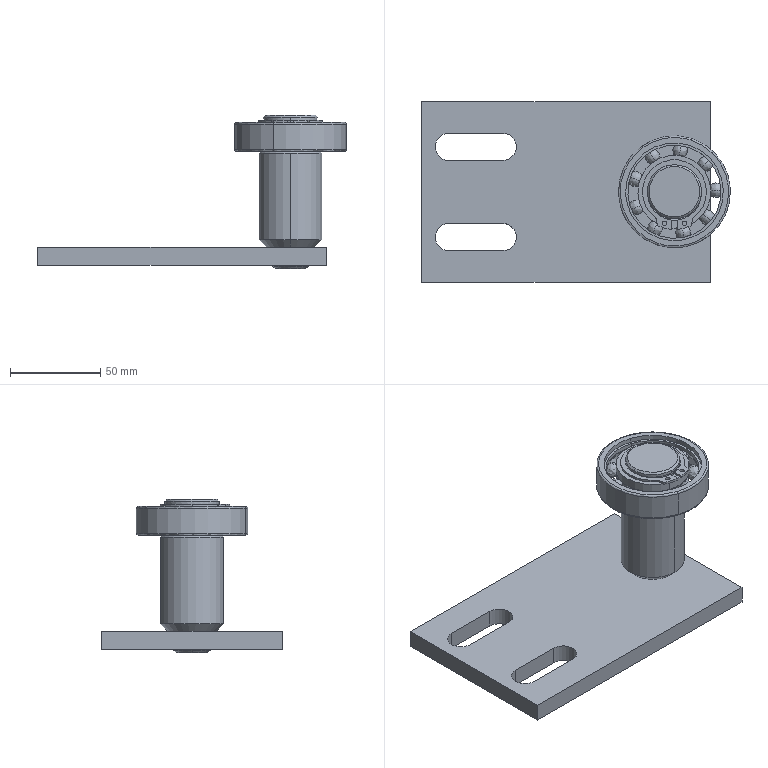Part | SolidWorks | features LayoutProfileFeature 1 | 3 solids | 122 faces | box 171 x 100 x 85 mm | volume 236433 mm3 | cylinder 50 | spline 36 | plane 28 | cone 8 | commonest cylinder face diameters 15 x6 30 x6 2.5 x4 20 x4 40.432 x4 51.568 x4